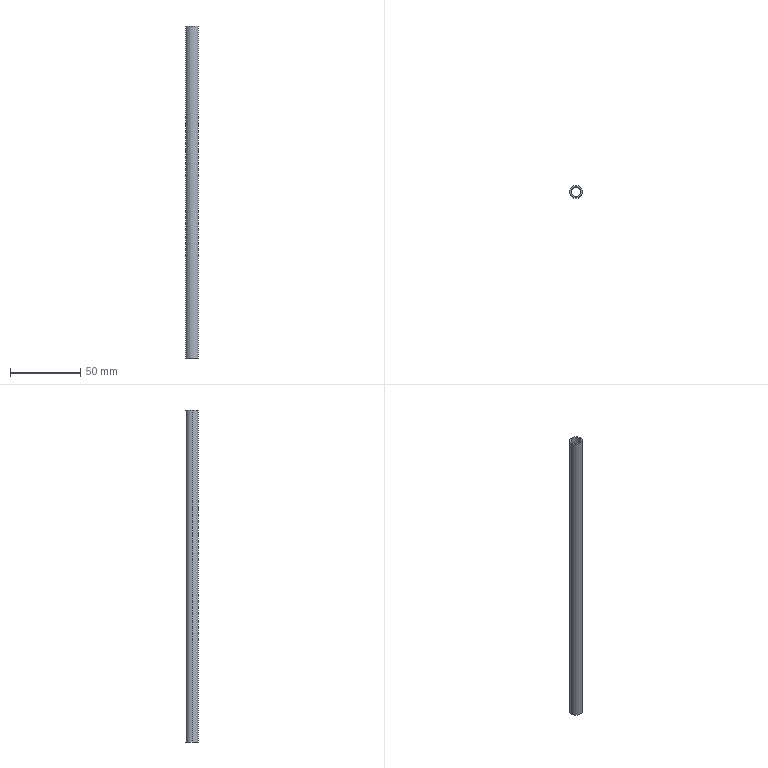Part | STEP file | DCV-000-019 | 1 solid | 6 faces | box 9 x 9 x 236 mm | volume 5931 mm3 | cylinder 4 | plane 2 | commonest cylinder face diameters 7 x2 9 x2
STEP:
#1=CARTESIAN_POINT('',(0.,0.,0.));
#2=DIRECTION('',(0.,0.,1.));
#3=DIRECTION('',(1.,0.,0.));
#4=AXIS2_PLACEMENT_3D('',#1,#2,#3);
#5=CARTESIAN_POINT('',(-3.5,0.,0.));
#6=VERTEX_POINT('',#5);
#7=CARTESIAN_POINT('',(-3.5,0.,236.));
#8=VERTEX_POINT('',#7);
#9=CARTESIAN_POINT('',(-3.5,0.,0.));
#10=DIRECTION('',(0.,0.,1.));
#11=VECTOR('',#10,1.);
#12=LINE('',#9,#11);
#13=CARTESIAN_POINT('',(0.,0.,0.));
#14=DIRECTION('',(0.,0.,1.));
#15=DIRECTION('',(-1.,0.,0.));
#16=AXIS2_PLACEMENT_3D('',#13,#14,#15);
#17=CYLINDRICAL_SURFACE('',#16,3.5);
#18=CARTESIAN_POINT('',(6.283,0.));
#19=DIRECTION('',(0.,1.));
#20=VECTOR('',#19,1.);
#21=LINE('',#18,#20);
#22=(GEOMETRIC_REPRESENTATION_CONTEXT(2)PARAMETRIC_REPRESENTATION_CONTEXT()REPRESENTATION_CONTEXT('',''));
#23=DEFINITIONAL_REPRESENTATION('',(#21),#22);
#24=PCURVE('',#17,#23);
#25=CARTESIAN_POINT('',(0.,0.,0.));
#26=DIRECTION('',(0.,0.,1.));
#27=DIRECTION('',(-1.,0.,0.));
#28=AXIS2_PLACEMENT_3D('',#25,#26,#27);
#29=CYLINDRICAL_SURFACE('',#28,3.5);
#30=CARTESIAN_POINT('',(0.,0.));
#31=DIRECTION('',(0.,1.));
#32=VECTOR('',#31,1.);
#33=LINE('',#30,#32);
#34=(GEOMETRIC_REPRESENTATION_CONTEXT(2)PARAMETRIC_REPRESENTATION_CONTEXT()REPRESENTATION_CONTEXT('',''));
#35=DEFINITIONAL_REPRESENTATION('',(#33),#34);
#36=PCURVE('',#29,#35);
#37=SURFACE_CURVE('',#12,(#24,#36),.PCURVE_S1.);
#38=EDGE_CURVE('',#6,#8,#37,.T.);
#39=ORIENTED_EDGE('',*,*,#38,.T.);
#40=CARTESIAN_POINT('',(3.5,0.,236.));
#41=VERTEX_POINT('',#40);
#42=CARTESIAN_POINT('',(0.,0.,236.));
#43=DIRECTION('',(0.,0.,-1.));
#44=DIRECTION('',(-1.,0.,0.));
#45=AXIS2_PLACEMENT_3D('',#42,#43,#44);
#46=CIRCLE('',#45,3.5);
#47=CARTESIAN_POINT('',(6.283,236.));
#48=DIRECTION('',(-1.,0.));
#49=VECTOR('',#48,1.);
#50=LINE('',#47,#49);
#51=(GEOMETRIC_REPRESENTATION_CONTEXT(2)PARAMETRIC_REPRESENTATION_CONTEXT()REPRESENTATION_CONTEXT('',''));
#52=DEFINITIONAL_REPRESENTATION('',(#50),#51);
#53=PCURVE('',#17,#52);
#54=CARTESIAN_POINT('',(0.,0.,236.));
#55=DIRECTION('',(0.,0.,1.));
#56=DIRECTION('',(1.,0.,0.));
#57=AXIS2_PLACEMENT_3D('',#54,#55,#56);
#58=PLANE('',#57);
#59=CARTESIAN_POINT('',(-3.5,0.));
#60=CARTESIAN_POINT('',(-3.5,6.062));
#61=CARTESIAN_POINT('',(1.75,3.031));
#62=CARTESIAN_POINT('',(7.,0.));
#63=CARTESIAN_POINT('',(1.75,-3.031));
#64=CARTESIAN_POINT('',(-3.5,-6.062));
#65=CARTESIAN_POINT('',(-3.5,0.));
#66=(BOUNDED_CURVE()B_SPLINE_CURVE(2,(#59,#60,#61,#62,#63,#64,#65),.UNSPECIFIED.,.T.,.F.)B_SPLINE_CURVE_WITH_KNOTS((1,2,2,2,2,1),(-2.094,0.,2.094,4.189,6.283,8.378),.UNSPECIFIED.)CURVE()GEOMETRIC_REPRESENTATION_ITEM()RATIONAL_B_SPLINE_CURVE((1.,0.5,1.,0.5,1.,0.5,1.))REPRESENTATION_ITEM(''));
#67=(GEOMETRIC_REPRESENTATION_CONTEXT(2)PARAMETRIC_REPRESENTATION_CONTEXT()REPRESENTATION_CONTEXT('',''));
#68=DEFINITIONAL_REPRESENTATION('',(#66),#67);
#69=PCURVE('',#58,#68);
#70=SURFACE_CURVE('',#46,(#53,#69),.PCURVE_S1.);
#71=EDGE_CURVE('',#8,#41,#70,.T.);
#72=ORIENTED_EDGE('',*,*,#71,.T.);
#73=CARTESIAN_POINT('',(3.5,0.,0.));
#74=VERTEX_POINT('',#73);
#75=CARTESIAN_POINT('',(3.5,0.,0.));
#76=DIRECTION('',(0.,0.,1.));
#77=VECTOR('',#76,1.);
#78=LINE('',#75,#77);
#79=CARTESIAN_POINT('',(3.142,0.));
#80=DIRECTION('',(0.,1.));
#81=VECTOR('',#80,1.);
#82=LINE('',#79,#81);
#83=(GEOMETRIC_REPRESENTATION_CONTEXT(2)PARAMETRIC_REPRESENTATION_CONTEXT()REPRESENTATION_CONTEXT('',''));
#84=DEFINITIONAL_REPRESENTATION('',(#82),#83);
#85=PCURVE('',#17,#84);
#86=CARTESIAN_POINT('',(3.142,0.));
#87=DIRECTION('',(0.,1.));
#88=VECTOR('',#87,1.);
#89=LINE('',#86,#88);
#90=(GEOMETRIC_REPRESENTATION_CONTEXT(2)PARAMETRIC_REPRESENTATION_CONTEXT()REPRESENTATION_CONTEXT('',''));
#91=DEFINITIONAL_REPRESENTATION('',(#89),#90);
#92=PCURVE('',#29,#91);
#93=SURFACE_CURVE('',#78,(#85,#92),.PCURVE_S1.);
#94=EDGE_CURVE('',#74,#41,#93,.T.);
#95=ORIENTED_EDGE('',*,*,#94,.F.);
#96=CARTESIAN_POINT('',(0.,0.,0.));
#97=DIRECTION('',(0.,0.,-1.));
#98=DIRECTION('',(-1.,0.,0.));
#99=AXIS2_PLACEMENT_3D('',#96,#97,#98);
#100=CIRCLE('',#99,3.5);
#101=CARTESIAN_POINT('',(6.283,0.));
#102=DIRECTION('',(-1.,0.));
#103=VECTOR('',#102,1.);
#104=LINE('',#101,#103);
#105=(GEOMETRIC_REPRESENTATION_CONTEXT(2)PARAMETRIC_REPRESENTATION_CONTEXT()REPRESENTATION_CONTEXT('',''));
#106=DEFINITIONAL_REPRESENTATION('',(#104),#105);
#107=PCURVE('',#17,#106);
#108=CARTESIAN_POINT('',(0.,0.,0.));
#109=DIRECTION('',(0.,0.,1.));
#110=DIRECTION('',(1.,0.,0.));
#111=AXIS2_PLACEMENT_3D('',#108,#109,#110);
#112=PLANE('',#111);
#113=CARTESIAN_POINT('',(-3.5,0.));
#114=CARTESIAN_POINT('',(-3.5,6.062));
#115=CARTESIAN_POINT('',(1.75,3.031));
#116=CARTESIAN_POINT('',(7.,0.));
#117=CARTESIAN_POINT('',(1.75,-3.031));
#118=CARTESIAN_POINT('',(-3.5,-6.062));
#119=CARTESIAN_POINT('',(-3.5,0.));
#120=(BOUNDED_CURVE()B_SPLINE_CURVE(2,(#113,#114,#115,#116,#117,#118,#119),.UNSPECIFIED.,.T.,.F.)B_SPLINE_CURVE_WITH_KNOTS((1,2,2,2,2,1),(-2.094,0.,2.094,4.189,6.283,8.378),.UNSPECIFIED.)CURVE()GEOMETRIC_REPRESENTATION_ITEM()RATIONAL_B_SPLINE_CURVE((1.,0.5,1.,0.5,1.,0.5,1.))REPRESENTATION_ITEM(''));
#121=(GEOMETRIC_REPRESENTATION_CONTEXT(2)PARAMETRIC_REPRESENTATION_CONTEXT()REPRESENTATION_CONTEXT('',''));
#122=DEFINITIONAL_REPRESENTATION('',(#120),#121);
#123=PCURVE('',#112,#122);
#124=SURFACE_CURVE('',#100,(#107,#123),.PCURVE_S1.);
#125=EDGE_CURVE('',#6,#74,#124,.T.);
#126=ORIENTED_EDGE('',*,*,#125,.F.);
#127=EDGE_LOOP('',(#39,#72,#95,#126));
#128=FACE_BOUND('',#127,.F.);
#129=ADVANCED_FACE('',(#128),#17,.F.);
#130=CARTESIAN_POINT('',(4.5,0.,0.));
#131=VERTEX_POINT('',#130);
#132=CARTESIAN_POINT('',(-4.5,0.,0.));
#133=VERTEX_POINT('',#132);
#134=CARTESIAN_POINT('',(0.,0.,0.));
#135=DIRECTION('',(0.,0.,1.));
#136=DIRECTION('',(1.,0.,0.));
#137=AXIS2_PLACEMENT_3D('',#134,#135,#136);
#138=CIRCLE('',#137,4.5);
#139=CARTESIAN_POINT('',(0.,0.,0.));
#140=DIRECTION('',(0.,0.,1.));
#141=DIRECTION('',(1.,0.,0.));
#142=AXIS2_PLACEMENT_3D('',#139,#140,#141);
#143=CYLINDRICAL_SURFACE('',#142,4.5);
#144=CARTESIAN_POINT('',(0.,0.));
#145=DIRECTION('',(1.,0.));
#146=VECTOR('',#145,1.);
#147=LINE('',#144,#146);
#148=(GEOMETRIC_REPRESENTATION_CONTEXT(2)PARAMETRIC_REPRESENTATION_CONTEXT()REPRESENTATION_CONTEXT('',''));
#149=DEFINITIONAL_REPRESENTATION('',(#147),#148);
#150=PCURVE('',#143,#149);
#151=CARTESIAN_POINT('',(0.,0.));
#152=DIRECTION('',(1.,0.));
#153=AXIS2_PLACEMENT_2D('',#151,#152);
#154=CIRCLE('',#153,4.5);
#155=(GEOMETRIC_REPRESENTATION_CONTEXT(2)PARAMETRIC_REPRESENTATION_CONTEXT()REPRESENTATION_CONTEXT('',''));
#156=DEFINITIONAL_REPRESENTATION('',(#154),#155);
#157=PCURVE('',#112,#156);
#158=SURFACE_CURVE('',#138,(#150,#157),.PCURVE_S1.);
#159=EDGE_CURVE('',#131,#133,#158,.T.);
#160=ORIENTED_EDGE('',*,*,#159,.T.);
#161=CARTESIAN_POINT('',(-4.5,0.,236.));
#162=VERTEX_POINT('',#161);
#163=CARTESIAN_POINT('',(-4.5,0.,0.));
#164=DIRECTION('',(0.,0.,1.));
#165=VECTOR('',#164,1.);
#166=LINE('',#163,#165);
#167=CARTESIAN_POINT('',(3.142,0.));
#168=DIRECTION('',(0.,1.));
#169=VECTOR('',#168,1.);
#170=LINE('',#167,#169);
#171=(GEOMETRIC_REPRESENTATION_CONTEXT(2)PARAMETRIC_REPRESENTATION_CONTEXT()REPRESENTATION_CONTEXT('',''));
#172=DEFINITIONAL_REPRESENTATION('',(#170),#171);
#173=PCURVE('',#143,#172);
#174=CARTESIAN_POINT('',(0.,0.,0.));
#175=DIRECTION('',(0.,0.,1.));
#176=DIRECTION('',(1.,0.,0.));
#177=AXIS2_PLACEMENT_3D('',#174,#175,#176);
#178=CYLINDRICAL_SURFACE('',#177,4.5);
#179=CARTESIAN_POINT('',(3.142,0.));
#180=DIRECTION('',(0.,1.));
#181=VECTOR('',#180,1.);
#182=LINE('',#179,#181);
#183=(GEOMETRIC_REPRESENTATION_CONTEXT(2)PARAMETRIC_REPRESENTATION_CONTEXT()REPRESENTATION_CONTEXT('',''));
#184=DEFINITIONAL_REPRESENTATION('',(#182),#183);
#185=PCURVE('',#178,#184);
#186=SURFACE_CURVE('',#166,(#173,#185),.PCURVE_S1.);
#187=EDGE_CURVE('',#133,#162,#186,.T.);
#188=ORIENTED_EDGE('',*,*,#187,.T.);
#189=CARTESIAN_POINT('',(4.5,0.,236.));
#190=VERTEX_POINT('',#189);
#191=CARTESIAN_POINT('',(0.,0.,236.));
#192=DIRECTION('',(0.,0.,1.));
#193=DIRECTION('',(1.,0.,0.));
#194=AXIS2_PLACEMENT_3D('',#191,#192,#193);
#195=CIRCLE('',#194,4.5);
#196=CARTESIAN_POINT('',(0.,236.));
#197=DIRECTION('',(1.,0.));
#198=VECTOR('',#197,1.);
#199=LINE('',#196,#198);
#200=(GEOMETRIC_REPRESENTATION_CONTEXT(2)PARAMETRIC_REPRESENTATION_CONTEXT()REPRESENTATION_CONTEXT('',''));
#201=DEFINITIONAL_REPRESENTATION('',(#199),#200);
#202=PCURVE('',#143,#201);
#203=CARTESIAN_POINT('',(0.,0.));
#204=DIRECTION('',(1.,0.));
#205=AXIS2_PLACEMENT_2D('',#203,#204);
#206=CIRCLE('',#205,4.5);
#207=(GEOMETRIC_REPRESENTATION_CONTEXT(2)PARAMETRIC_REPRESENTATION_CONTEXT()REPRESENTATION_CONTEXT('',''));
#208=DEFINITIONAL_REPRESENTATION('',(#206),#207);
#209=PCURVE('',#58,#208);
#210=SURFACE_CURVE('',#195,(#202,#209),.PCURVE_S1.);
#211=EDGE_CURVE('',#190,#162,#210,.T.);
#212=ORIENTED_EDGE('',*,*,#211,.F.);
#213=CARTESIAN_POINT('',(4.5,0.,0.));
#214=DIRECTION('',(0.,0.,1.));
#215=VECTOR('',#214,1.);
#216=LINE('',#213,#215);
#217=CARTESIAN_POINT('',(0.,0.));
#218=DIRECTION('',(0.,1.));
#219=VECTOR('',#218,1.);
#220=LINE('',#217,#219);
#221=(GEOMETRIC_REPRESENTATION_CONTEXT(2)PARAMETRIC_REPRESENTATION_CONTEXT()REPRESENTATION_CONTEXT('',''));
#222=DEFINITIONAL_REPRESENTATION('',(#220),#221);
#223=PCURVE('',#143,#222);
#224=CARTESIAN_POINT('',(6.283,0.));
#225=DIRECTION('',(0.,1.));
#226=VECTOR('',#225,1.);
#227=LINE('',#224,#226);
#228=(GEOMETRIC_REPRESENTATION_CONTEXT(2)PARAMETRIC_REPRESENTATION_CONTEXT()REPRESENTATION_CONTEXT('',''));
#229=DEFINITIONAL_REPRESENTATION('',(#227),#228);
#230=PCURVE('',#178,#229);
#231=SURFACE_CURVE('',#216,(#223,#230),.PCURVE_S1.);
#232=EDGE_CURVE('',#131,#190,#231,.T.);
#233=ORIENTED_EDGE('',*,*,#232,.F.);
#234=EDGE_LOOP('',(#160,#188,#212,#233));
#235=FACE_BOUND('',#234,.T.);
#236=ADVANCED_FACE('',(#235),#143,.T.);
#237=ORIENTED_EDGE('',*,*,#125,.F.);
#238=CARTESIAN_POINT('',(0.,0.,0.));
#239=DIRECTION('',(0.,0.,-1.));
#240=DIRECTION('',(-1.,0.,0.));
#241=AXIS2_PLACEMENT_3D('',#238,#239,#240);
#242=CIRCLE('',#241,3.5);
#243=CARTESIAN_POINT('',(-3.5,0.));
#244=CARTESIAN_POINT('',(-3.5,6.062));
#245=CARTESIAN_POINT('',(1.75,3.031));
#246=CARTESIAN_POINT('',(7.,0.));
#247=CARTESIAN_POINT('',(1.75,-3.031));
#248=CARTESIAN_POINT('',(-3.5,-6.062));
#249=CARTESIAN_POINT('',(-3.5,0.));
#250=(BOUNDED_CURVE()B_SPLINE_CURVE(2,(#243,#244,#245,#246,#247,#248,#249),.UNSPECIFIED.,.T.,.F.)B_SPLINE_CURVE_WITH_KNOTS((1,2,2,2,2,1),(-2.094,0.,2.094,4.189,6.283,8.378),.UNSPECIFIED.)CURVE()GEOMETRIC_REPRESENTATION_ITEM()RATIONAL_B_SPLINE_CURVE((1.,0.5,1.,0.5,1.,0.5,1.))REPRESENTATION_ITEM(''));
#251=(GEOMETRIC_REPRESENTATION_CONTEXT(2)PARAMETRIC_REPRESENTATION_CONTEXT()REPRESENTATION_CONTEXT('',''));
#252=DEFINITIONAL_REPRESENTATION('',(#250),#251);
#253=PCURVE('',#112,#252);
#254=CARTESIAN_POINT('',(6.283,0.));
#255=DIRECTION('',(-1.,0.));
#256=VECTOR('',#255,1.);
#257=LINE('',#254,#256);
#258=(GEOMETRIC_REPRESENTATION_CONTEXT(2)PARAMETRIC_REPRESENTATION_CONTEXT()REPRESENTATION_CONTEXT('',''));
#259=DEFINITIONAL_REPRESENTATION('',(#257),#258);
#260=PCURVE('',#29,#259);
#261=SURFACE_CURVE('',#242,(#253,#260),.PCURVE_S1.);
#262=EDGE_CURVE('',#74,#6,#261,.T.);
#263=ORIENTED_EDGE('',*,*,#262,.F.);
#264=EDGE_LOOP('',(#237,#263));
#265=FACE_BOUND('',#264,.T.);
#266=ORIENTED_EDGE('',*,*,#159,.F.);
#267=CARTESIAN_POINT('',(0.,0.,0.));
#268=DIRECTION('',(0.,0.,1.));
#269=DIRECTION('',(1.,0.,0.));
#270=AXIS2_PLACEMENT_3D('',#267,#268,#269);
#271=CIRCLE('',#270,4.5);
#272=CARTESIAN_POINT('',(0.,0.));
#273=DIRECTION('',(1.,0.));
#274=AXIS2_PLACEMENT_2D('',#272,#273);
#275=CIRCLE('',#274,4.5);
#276=(GEOMETRIC_REPRESENTATION_CONTEXT(2)PARAMETRIC_REPRESENTATION_CONTEXT()REPRESENTATION_CONTEXT('',''));
#277=DEFINITIONAL_REPRESENTATION('',(#275),#276);
#278=PCURVE('',#112,#277);
#279=CARTESIAN_POINT('',(0.,0.));
#280=DIRECTION('',(1.,0.));
#281=VECTOR('',#280,1.);
#282=LINE('',#279,#281);
#283=(GEOMETRIC_REPRESENTATION_CONTEXT(2)PARAMETRIC_REPRESENTATION_CONTEXT()REPRESENTATION_CONTEXT('',''));
#284=DEFINITIONAL_REPRESENTATION('',(#282),#283);
#285=PCURVE('',#178,#284);
#286=SURFACE_CURVE('',#271,(#278,#285),.PCURVE_S1.);
#287=EDGE_CURVE('',#133,#131,#286,.T.);
#288=ORIENTED_EDGE('',*,*,#287,.F.);
#289=EDGE_LOOP('',(#266,#288));
#290=FACE_BOUND('',#289,.T.);
#291=ADVANCED_FACE('',(#265,#290),#112,.F.);
#292=ORIENTED_EDGE('',*,*,#71,.T.);
#293=CARTESIAN_POINT('',(0.,0.,236.));
#294=DIRECTION('',(0.,0.,-1.));
#295=DIRECTION('',(-1.,0.,0.));
#296=AXIS2_PLACEMENT_3D('',#293,#294,#295);
#297=CIRCLE('',#296,3.5);
#298=CARTESIAN_POINT('',(-3.5,0.));
#299=CARTESIAN_POINT('',(-3.5,6.062));
#300=CARTESIAN_POINT('',(1.75,3.031));
#301=CARTESIAN_POINT('',(7.,0.));
#302=CARTESIAN_POINT('',(1.75,-3.031));
#303=CARTESIAN_POINT('',(-3.5,-6.062));
#304=CARTESIAN_POINT('',(-3.5,0.));
#305=(BOUNDED_CURVE()B_SPLINE_CURVE(2,(#298,#299,#300,#301,#302,#303,#304),.UNSPECIFIED.,.T.,.F.)B_SPLINE_CURVE_WITH_KNOTS((1,2,2,2,2,1),(-2.094,0.,2.094,4.189,6.283,8.378),.UNSPECIFIED.)CURVE()GEOMETRIC_REPRESENTATION_ITEM()RATIONAL_B_SPLINE_CURVE((1.,0.5,1.,0.5,1.,0.5,1.))REPRESENTATION_ITEM(''));
#306=(GEOMETRIC_REPRESENTATION_CONTEXT(2)PARAMETRIC_REPRESENTATION_CONTEXT()REPRESENTATION_CONTEXT('',''));
#307=DEFINITIONAL_REPRESENTATION('',(#305),#306);
#308=PCURVE('',#58,#307);
#309=CARTESIAN_POINT('',(6.283,236.));
#310=DIRECTION('',(-1.,0.));
#311=VECTOR('',#310,1.);
#312=LINE('',#309,#311);
#313=(GEOMETRIC_REPRESENTATION_CONTEXT(2)PARAMETRIC_REPRESENTATION_CONTEXT()REPRESENTATION_CONTEXT('',''));
#314=DEFINITIONAL_REPRESENTATION('',(#312),#313);
#315=PCURVE('',#29,#314);
#316=SURFACE_CURVE('',#297,(#308,#315),.PCURVE_S1.);
#317=EDGE_CURVE('',#41,#8,#316,.T.);
#318=ORIENTED_EDGE('',*,*,#317,.T.);
#319=EDGE_LOOP('',(#292,#318));
#320=FACE_BOUND('',#319,.T.);
#321=ORIENTED_EDGE('',*,*,#211,.T.);
#322=CARTESIAN_POINT('',(0.,0.,236.));
#323=DIRECTION('',(0.,0.,1.));
#324=DIRECTION('',(1.,0.,0.));
#325=AXIS2_PLACEMENT_3D('',#322,#323,#324);
#326=CIRCLE('',#325,4.5);
#327=CARTESIAN_POINT('',(0.,0.));
#328=DIRECTION('',(1.,0.));
#329=AXIS2_PLACEMENT_2D('',#327,#328);
#330=CIRCLE('',#329,4.5);
#331=(GEOMETRIC_REPRESENTATION_CONTEXT(2)PARAMETRIC_REPRESENTATION_CONTEXT()REPRESENTATION_CONTEXT('',''));
#332=DEFINITIONAL_REPRESENTATION('',(#330),#331);
#333=PCURVE('',#58,#332);
#334=CARTESIAN_POINT('',(0.,236.));
#335=DIRECTION('',(1.,0.));
#336=VECTOR('',#335,1.);
#337=LINE('',#334,#336);
#338=(GEOMETRIC_REPRESENTATION_CONTEXT(2)PARAMETRIC_REPRESENTATION_CONTEXT()REPRESENTATION_CONTEXT('',''));
#339=DEFINITIONAL_REPRESENTATION('',(#337),#338);
#340=PCURVE('',#178,#339);
#341=SURFACE_CURVE('',#326,(#333,#340),.PCURVE_S1.);
#342=EDGE_CURVE('',#162,#190,#341,.T.);
#343=ORIENTED_EDGE('',*,*,#342,.T.);
#344=EDGE_LOOP('',(#321,#343));
#345=FACE_BOUND('',#344,.T.);
#346=ADVANCED_FACE('',(#320,#345),#58,.T.);
#347=ORIENTED_EDGE('',*,*,#187,.F.);
#348=ORIENTED_EDGE('',*,*,#287,.T.);
#349=ORIENTED_EDGE('',*,*,#232,.T.);
#350=ORIENTED_EDGE('',*,*,#342,.F.);
#351=EDGE_LOOP('',(#347,#348,#349,#350));
#352=FACE_BOUND('',#351,.T.);
#353=ADVANCED_FACE('',(#352),#178,.T.);
#354=ORIENTED_EDGE('',*,*,#317,.T.);
#355=ORIENTED_EDGE('',*,*,#38,.F.);
#356=ORIENTED_EDGE('',*,*,#262,.F.);
#357=ORIENTED_EDGE('',*,*,#94,.T.);
#358=EDGE_LOOP('',(#354,#355,#356,#357));
#359=FACE_BOUND('',#358,.F.);
#360=ADVANCED_FACE('',(#359),#29,.F.);
#361=CLOSED_SHELL('',(#129,#236,#291,#346,#353,#360));
#362=MANIFOLD_SOLID_BREP('',#361);
#363=(LENGTH_UNIT()NAMED_UNIT(*)SI_UNIT(.MILLI.,.METRE.));
#364=UNCERTAINTY_MEASURE_WITH_UNIT(LENGTH_MEASURE(0.0000001),#363,'','');
#365=(NAMED_UNIT(*)PLANE_ANGLE_UNIT()SI_UNIT($,.RADIAN.));
#366=(NAMED_UNIT(*)SI_UNIT($,.STERADIAN.)SOLID_ANGLE_UNIT());
#367=(GEOMETRIC_REPRESENTATION_CONTEXT(3)GLOBAL_UNCERTAINTY_ASSIGNED_CONTEXT((#364))GLOBAL_UNIT_ASSIGNED_CONTEXT((#363,#365,#366))REPRESENTATION_CONTEXT('',''));
#368=ADVANCED_BREP_SHAPE_REPRESENTATION('',(#4,#362),#367);